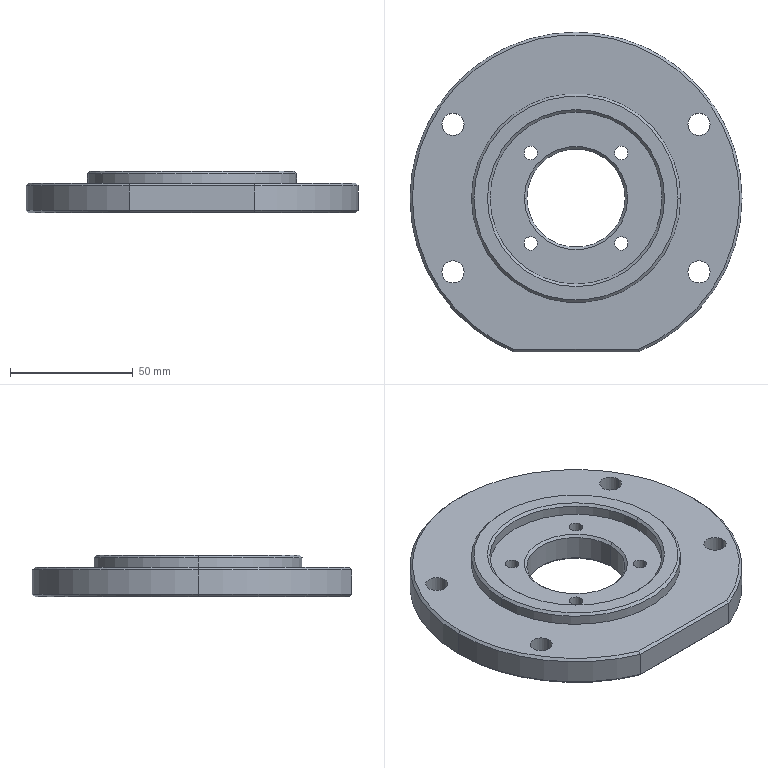Part | STEP file | YCD14007A-08.03.07.05 Adapter Flange (Motor) | 1 solid | 46 faces | box 135 x 130 x 17 mm | volume 158776 mm3 | cylinder 25 | cone 14 | plane 7 | commonest cylinder face diameters 5.5 x8 9 x8 135 x3 40 x2 70 x2 85 x2